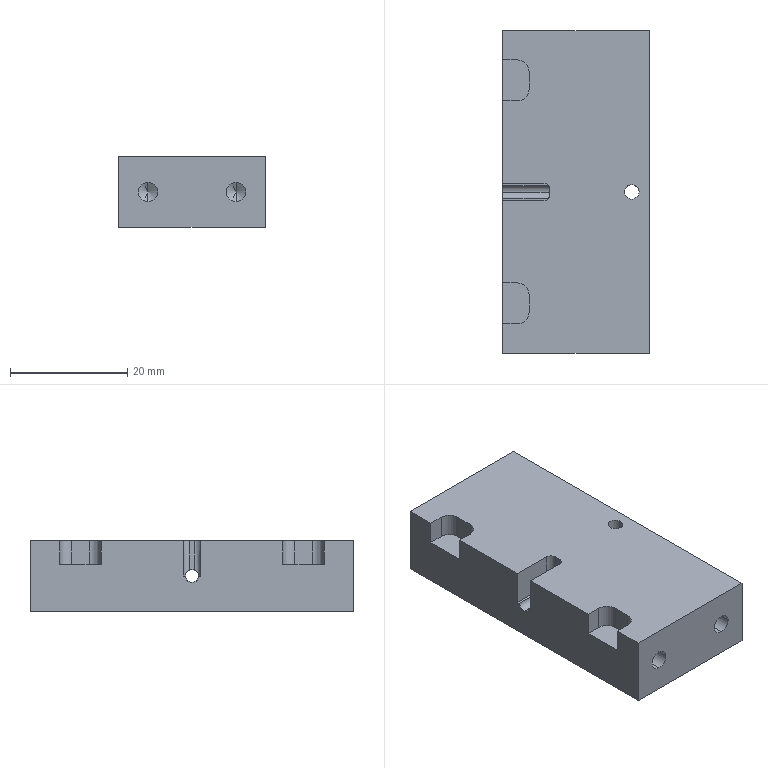Part | SolidWorks | features ICE 4, Chamfer 2, Fillet 2, HoleWzd 2, MirrorPattern 2, Extrusion 1 | 1 solid | 52 faces | box 25 x 55 x 12 mm | volume 15520 mm3 | cylinder 22 | plane 20 | cone 8 | torus 2 | commonest cylinder face diameters 3.3 x8 2.5 x4 4 x4 2 x2 2.2 x2 5 x2